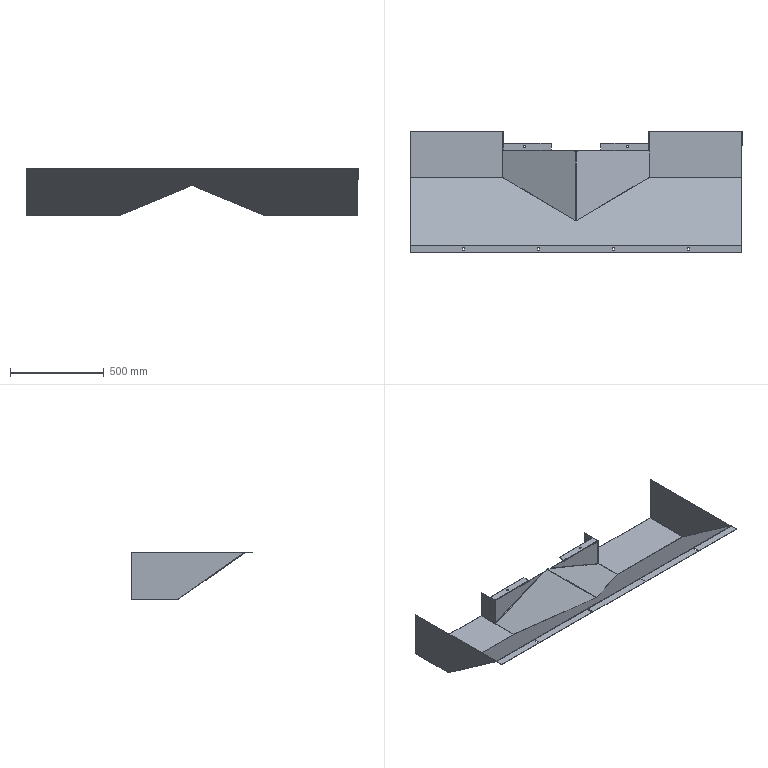Part | SolidWorks | features BaseBody 4 | 4 solids | 151 faces | box 1770 x 649.052 x 254.655 mm | volume 3040079 mm3 | plane 108 | cylinder 34 | spline 9 | commonest cylinder face diameters 7 x14 2 x10 6 x10